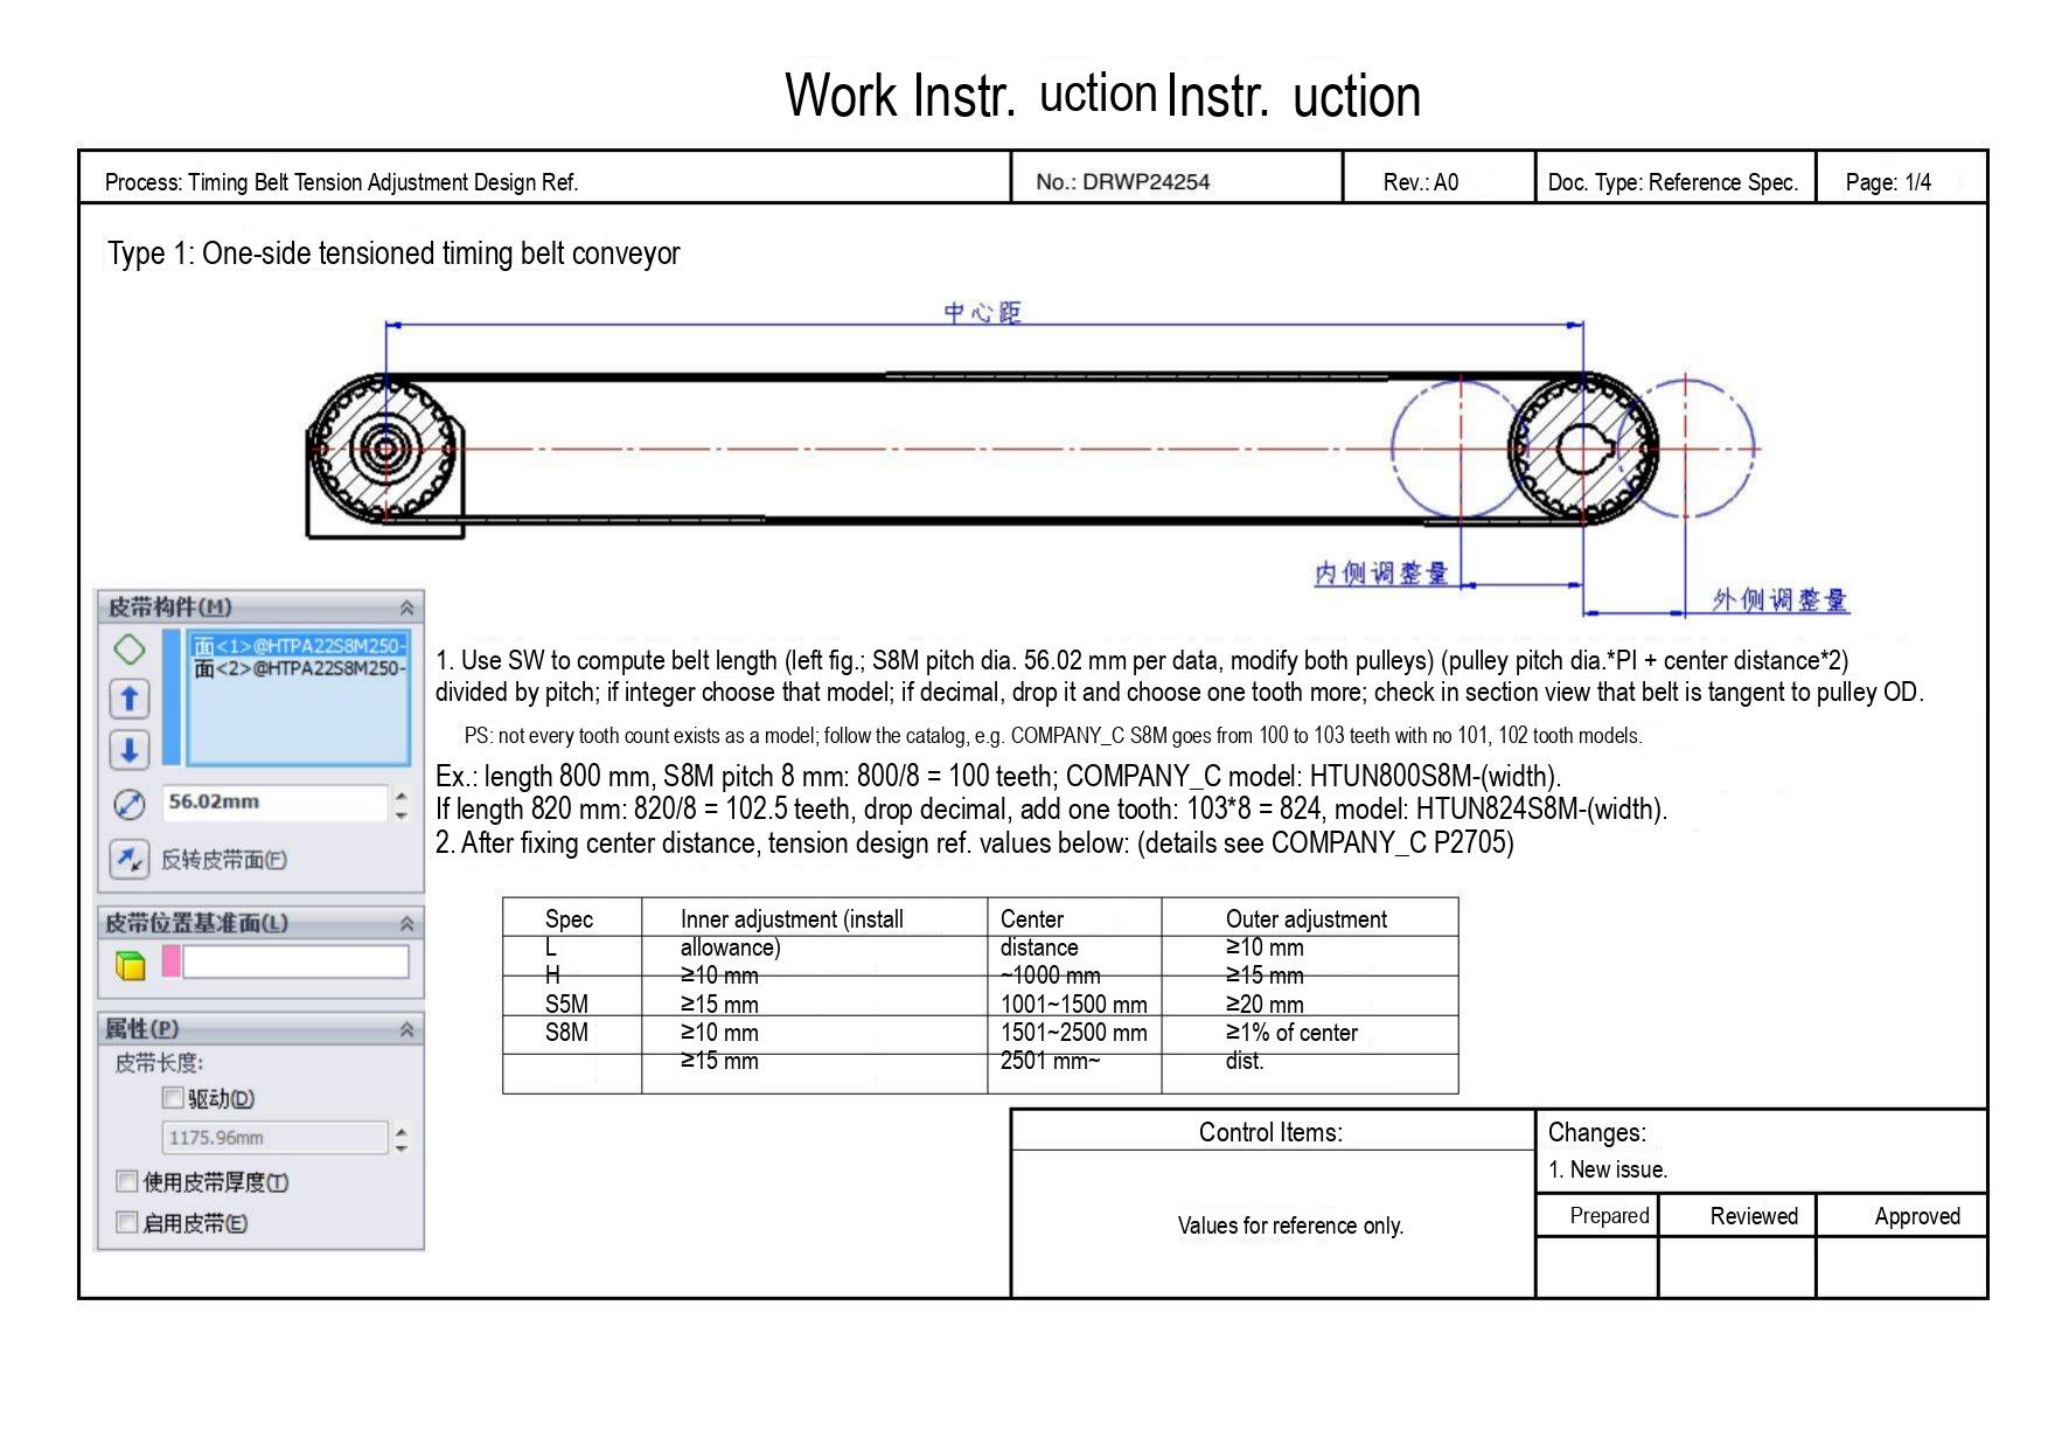# Work Instr. uction Instr. uction

| Process: Timing Belt Tension Adjustment Design Ref. | No.: DRWP24254 | Rev.: A0 | Doc. Type: Reference Spec. | Page: 1/4 |
|---|---|---|---|---|

Type 1: One-side tensioned timing belt conveyor

中心距

内侧调整量

外侧调整量

皮带构件(M)

面<1>@HTPA22S8M250-
面<2>@HTPA22S8M250-

56.02mm

反转皮带面(F)

皮带位置基准面(L)

属性(P)

皮带长度:

驱动(D)

1175.96mm

使用皮带厚度(T)

启用皮带(E)

1. Use SW to compute belt length (left fig.; S8M pitch dia. 56.02 mm per data, modify both pulleys) (pulley pitch dia.*PI + center distance*2) divided by pitch; if integer choose that model; if decimal, drop it and choose one tooth more; check in section view that belt is tangent to pulley OD.

PS: not every tooth count exists as a model; follow the catalog, e.g. COMPANY_C S8M goes from 100 to 103 teeth with no 101, 102 tooth models.

Ex.: length 800 mm, S8M pitch 8 mm: 800/8 = 100 teeth; COMPANY_C model: HTUN800S8M-(width).
If length 820 mm: 820/8 = 102.5 teeth, drop decimal, add one tooth: 103*8 = 824, model: HTUN824S8M-(width).
2. After fixing center distance, tension design ref. values below: (details see COMPANY_C P2705)

| Spec | Inner adjustment (install | Center | Outer adjustment |
|---|---|---|---|
| L | allowance) | distance | ≥10 mm |
| H | ≥10 mm | ~1000 mm | ≥15 mm |
| S5M | ≥15 mm | 1001~1500 mm | ≥20 mm |
| S8M | ≥10 mm | 1501~2500 mm | ≥1% of center |
| | ≥15 mm | 2501 mm~ | dist. |

| Control Items: | Changes: | | |
|---|---|---|---|
| | 1. New issue. | | |
| Values for reference only. | Prepared | Reviewed | Approved |
| | | | |
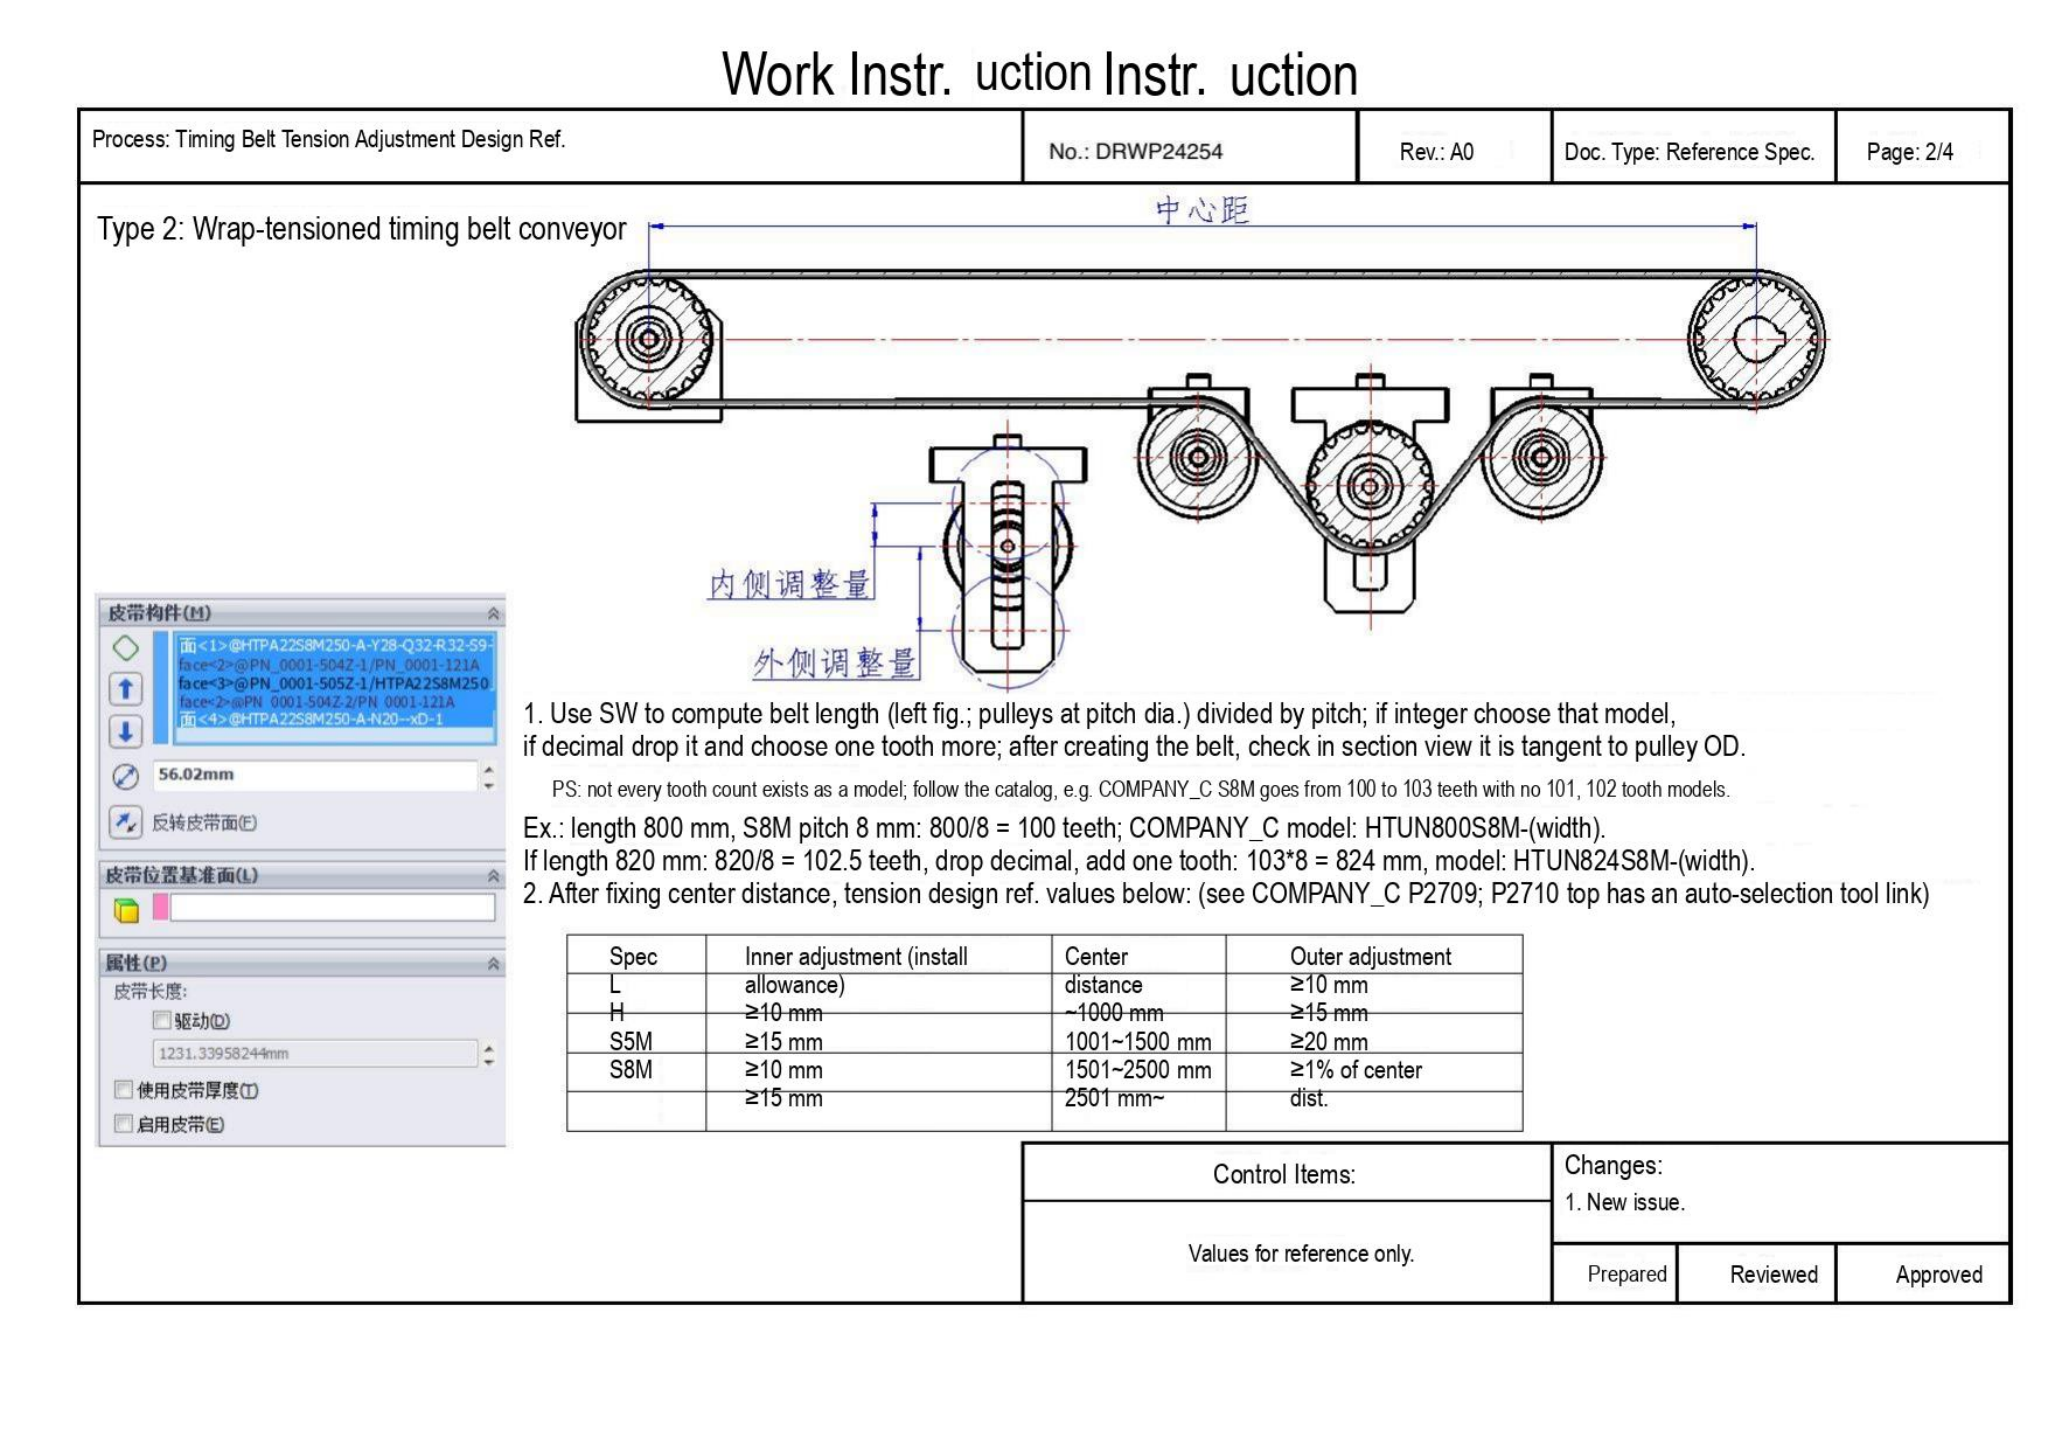# Work Instr. uction Instr. uction

| Process: Timing Belt Tension Adjustment Design Ref. | No.: DRWP24254 | Rev.: A0 | Doc. Type: Reference Spec. | Page: 2/4 |
|---|---|---|---|---|

Type 2: Wrap-tensioned timing belt conveyor

中心距

内侧调整量

外侧调整量

皮带构件(M)

面<1>@HTPA22S8M250-A-Y28-Q32-R32-S9-
face<2>@PN_0001-504Z-1/PN_0001-121A
face<3>@PN_0001-505Z-1/HTPA22S8M250
face<2>@PN_0001-504Z-2/PN_0001-121A
面<4>@HTPA22S8M250-A-N20--xD-1

56.02mm

反转皮带面(F)

皮带位置基准面(L)

属性(P)

皮带长度:

驱动(D)

1231.33958244mm

使用皮带厚度(T)

启用皮带(E)

1. Use SW to compute belt length (left fig.; pulleys at pitch dia.) divided by pitch; if integer choose that model, if decimal drop it and choose one tooth more; after creating the belt, check in section view it is tangent to pulley OD.

PS: not every tooth count exists as a model; follow the catalog, e.g. COMPANY_C S8M goes from 100 to 103 teeth with no 101, 102 tooth models.

Ex.: length 800 mm, S8M pitch 8 mm: 800/8 = 100 teeth; COMPANY_C model: HTUN800S8M-(width).
If length 820 mm: 820/8 = 102.5 teeth, drop decimal, add one tooth: 103*8 = 824 mm, model: HTUN824S8M-(width).
2. After fixing center distance, tension design ref. values below: (see COMPANY_C P2709; P2710 top has an auto-selection tool link)

| Spec | Inner adjustment (install | Center | Outer adjustment |
|---|---|---|---|
| L | allowance) | distance | ≥10 mm |
| H | ≥10 mm | ~1000 mm | ≥15 mm |
| S5M | ≥15 mm | 1001~1500 mm | ≥20 mm |
| S8M | ≥10 mm | 1501~2500 mm | ≥1% of center |
| | ≥15 mm | 2501 mm~ | dist. |

| Control Items: | Changes: 1. New issue. | | |
|---|---|---|---|
| Values for reference only. | Prepared | Reviewed | Approved |
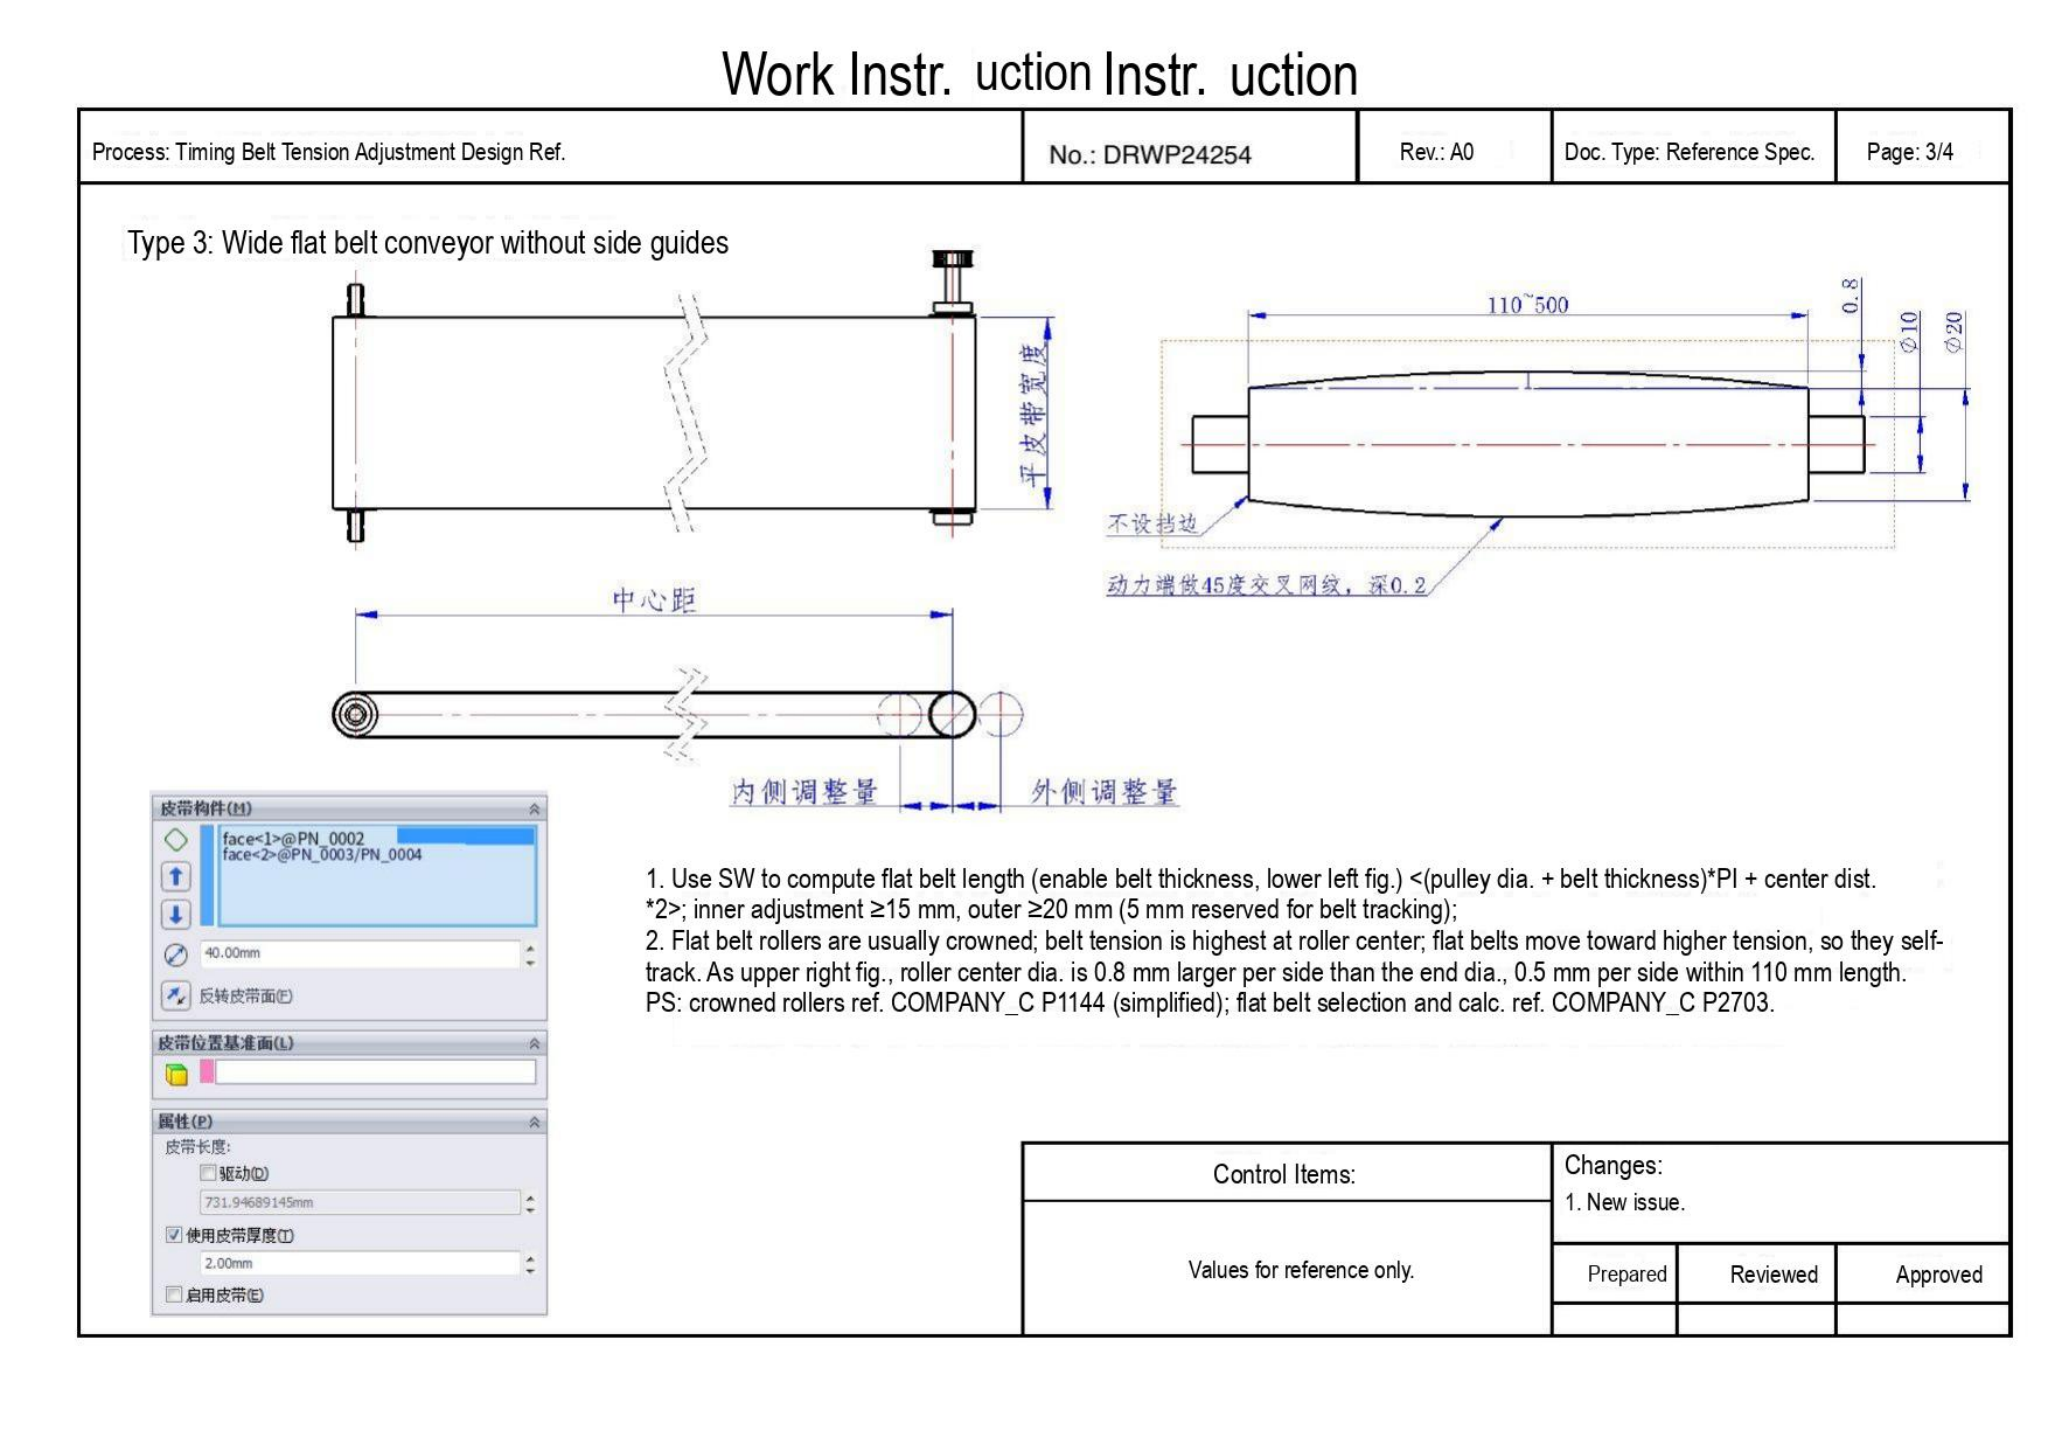Work Instr. uction Instr. uction

| Process: Timing Belt Tension Adjustment Design Ref. | No.: DRWP24254 | Rev.: A0 | Doc. Type: Reference Spec. | Page: 3/4 |
|---|---|---|---|---|

Type 3: Wide flat belt conveyor without side guides

平皮带宽度

110~500

0.8

Ø10

Ø20

不设挡边

动力端做45度交叉网纹，深0.2

中心距

内侧调整量

外侧调整量

皮带构件(M)

face<1>@PN_0002
face<2>@PN_0003/PN_0004

40.00mm

反转皮带面(E)

皮带位置基准面(L)

属性(P)

皮带长度:

驱动(D)

731.94689145mm

使用皮带厚度(T)

2.00mm

启用皮带(E)

1. Use SW to compute flat belt length (enable belt thickness, lower left fig.) <(pulley dia. + belt thickness)*PI + center dist. *2>; inner adjustment ≥15 mm, outer ≥20 mm (5 mm reserved for belt tracking);
2. Flat belt rollers are usually crowned; belt tension is highest at roller center; flat belts move toward higher tension, so they self-track. As upper right fig., roller center dia. is 0.8 mm larger per side than the end dia., 0.5 mm per side within 110 mm length.
PS: crowned rollers ref. COMPANY_C P1144 (simplified); flat belt selection and calc. ref. COMPANY_C P2703.

| Control Items: | Changes: 1. New issue. | | |
|---|---|---|---|
| Values for reference only. | Prepared | Reviewed | Approved |
| | | | |
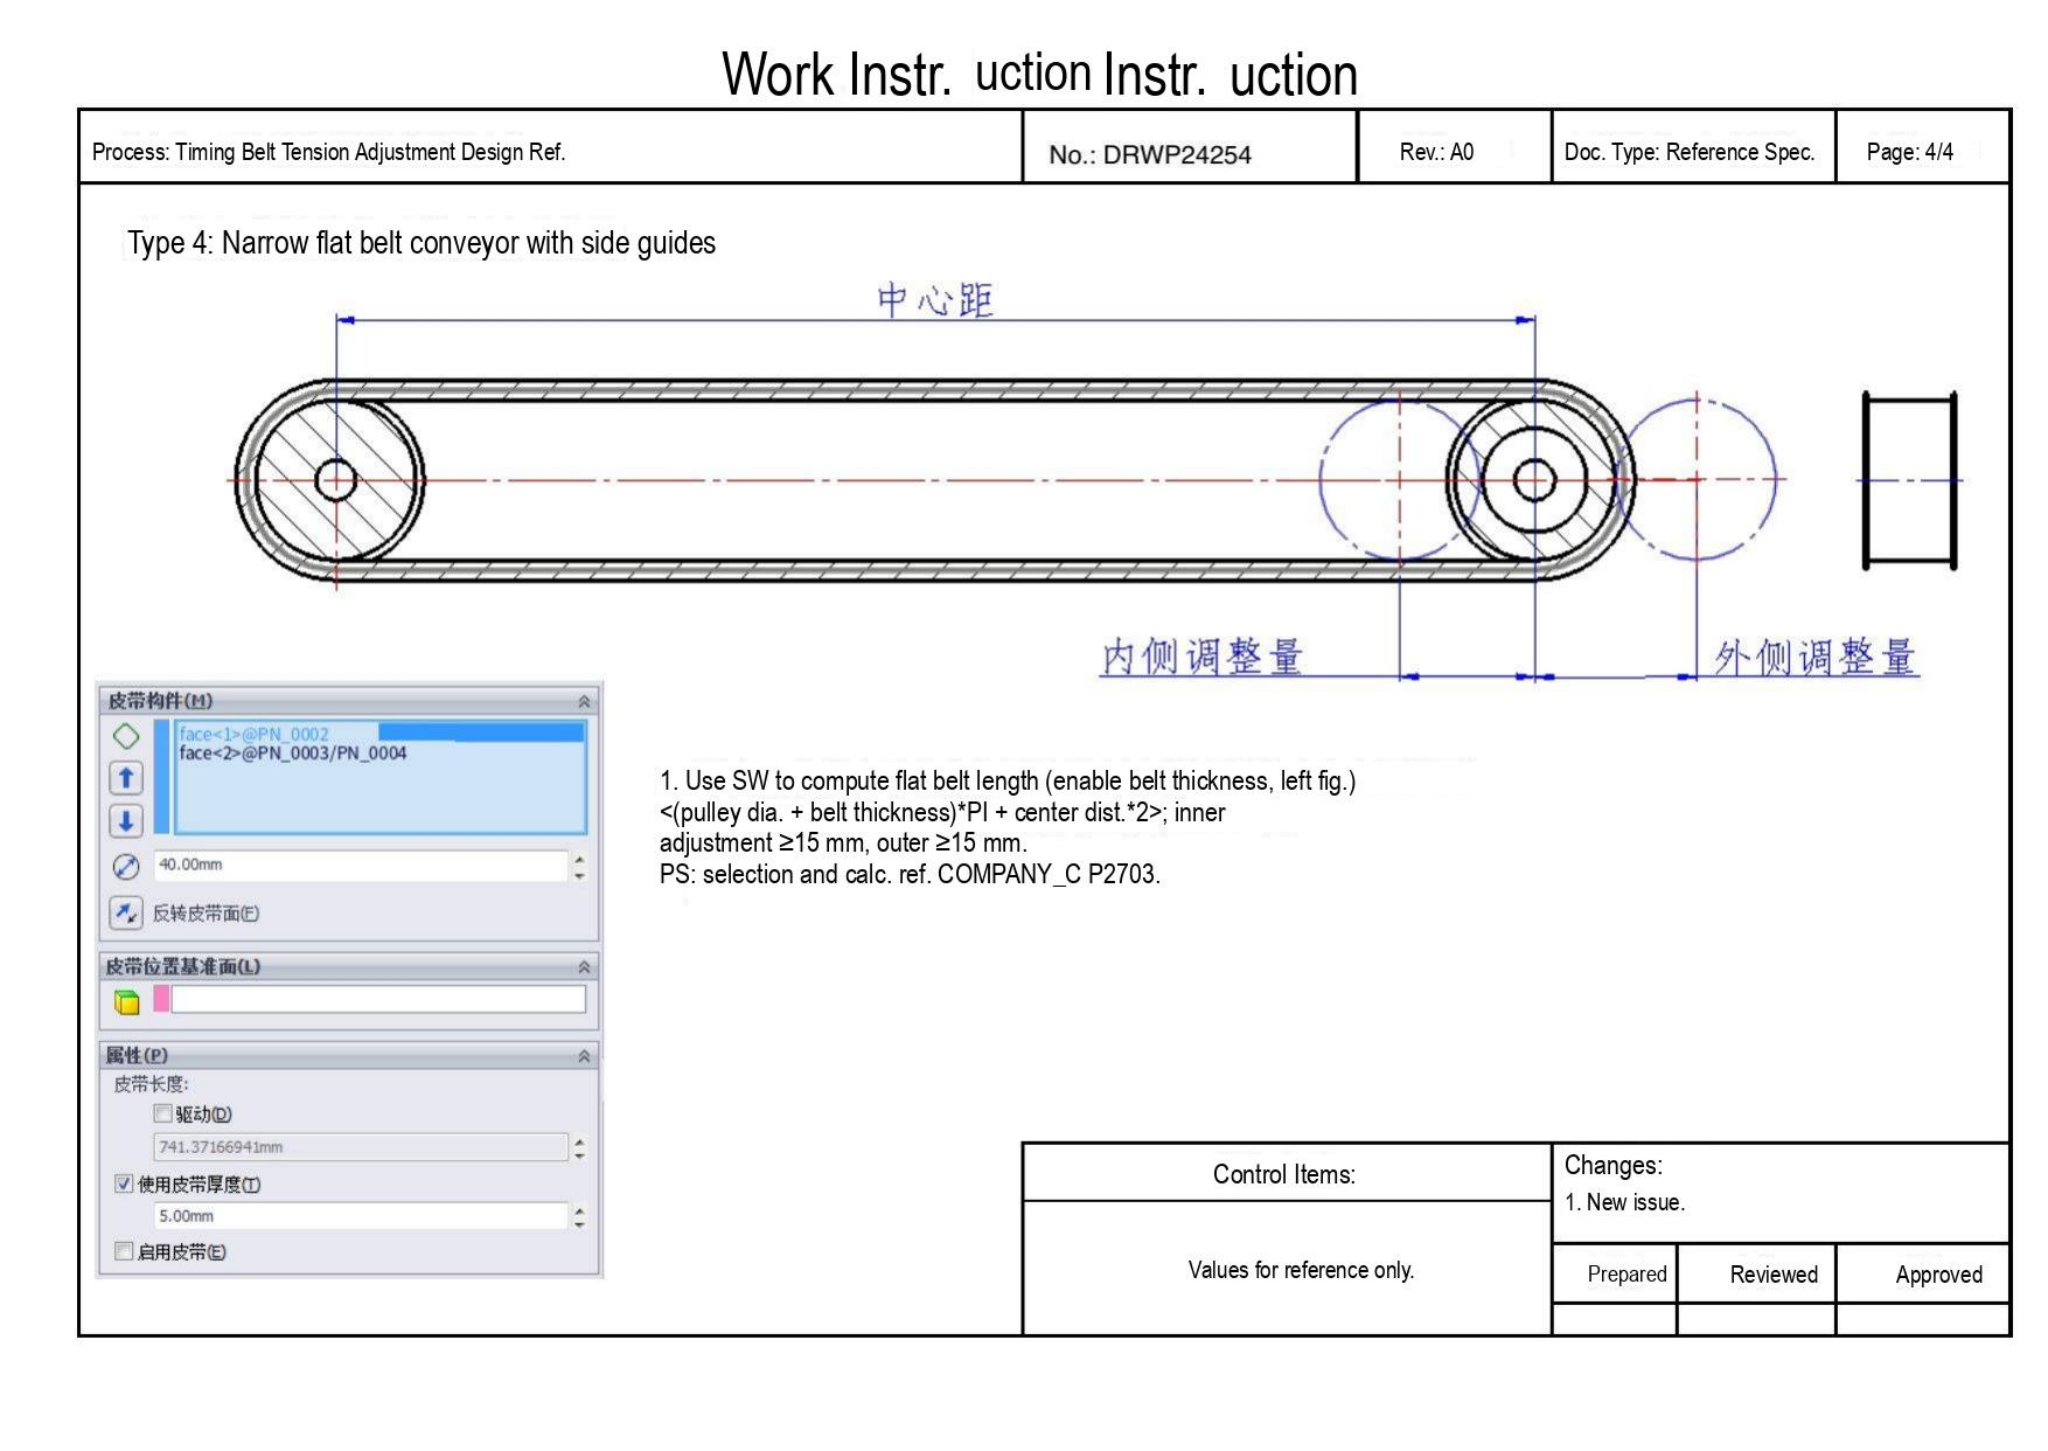Work Instr. uction Instr. uction

| Process: Timing Belt Tension Adjustment Design Ref. | No.: DRWP24254 | Rev.: A0 | Doc. Type: Reference Spec. | Page: 4/4 |
|---|---|---|---|---|

Type 4: Narrow flat belt conveyor with side guides

中心距

内侧调整量

外侧调整量

皮带构件(M)

face<1>@PN_0002
face<2>@PN_0003/PN_0004

40.00mm

反转皮带面(F)

皮带位置基准面(L)

属性(P)

皮带长度:

驱动(D)

741.37166941mm

使用皮带厚度(T)

5.00mm

启用皮带(E)

1. Use SW to compute flat belt length (enable belt thickness, left fig.)
<(pulley dia. + belt thickness)*PI + center dist.*2>; inner
adjustment ≥15 mm, outer ≥15 mm.
PS: selection and calc. ref. COMPANY_C P2703.

| Control Items: | Changes: 1. New issue. | | |
|---|---|---|---|
| Values for reference only. | Prepared | Reviewed | Approved |
| | | | |